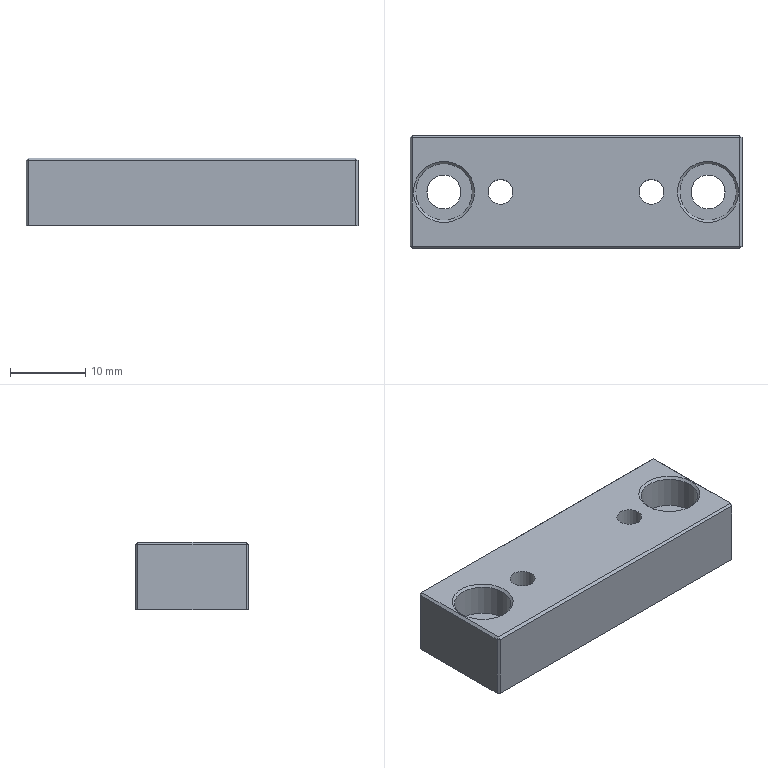Part | NX | 1 solid | 28 faces | box 44 x 15 x 9 mm | volume 5236 mm3 | plane 20 | cylinder 6 | cone 2 | commonest cylinder face diameters 3.3 x2 4.5 x2 7.5 x2
STEP:
#1=CARTESIAN_POINT('',(-106.55,-217.899,185.));
#2=VERTEX_POINT('',#1);
#3=CARTESIAN_POINT('',(-102.5,-217.899,185.));
#4=DIRECTION('',(0.,0.,-1.));
#5=DIRECTION('',(-1.,0.,0.));
#6=AXIS2_PLACEMENT_3D('',#3,#4,#5);
#7=CIRCLE('',#6,4.05);
#8=EDGE_CURVE('',#2,#2,#7,.T.);
#9=ORIENTED_EDGE('',*,*,#8,.F.);
#10=EDGE_LOOP('',(#9));
#11=FACE_BOUND('',#10,.T.);
#12=CARTESIAN_POINT('',(-106.25,-217.899,184.7));
#13=VERTEX_POINT('',#12);
#14=CARTESIAN_POINT('',(-102.5,-217.899,184.7));
#15=DIRECTION('',(0.,0.,1.));
#16=DIRECTION('',(-1.,0.,0.));
#17=AXIS2_PLACEMENT_3D('',#14,#15,#16);
#18=CIRCLE('',#17,3.75);
#19=EDGE_CURVE('',#13,#13,#18,.T.);
#20=ORIENTED_EDGE('',*,*,#19,.F.);
#21=EDGE_LOOP('',(#20));
#22=FACE_BOUND('',#21,.T.);
#23=CARTESIAN_POINT('',(-102.5,-217.899,185.));
#24=DIRECTION('',(0.,0.,1.));
#25=DIRECTION('',(1.,0.,0.));
#26=AXIS2_PLACEMENT_3D('',#23,#24,#25);
#27=CONICAL_SURFACE('',#26,4.05,0.7854);
#28=ADVANCED_FACE('',(#11,#22),#27,.F.);
#29=CARTESIAN_POINT('',(-71.55,-217.899,185.));
#30=VERTEX_POINT('',#29);
#31=CARTESIAN_POINT('',(-67.5,-217.899,185.));
#32=DIRECTION('',(0.,0.,-1.));
#33=DIRECTION('',(-1.,0.,0.));
#34=AXIS2_PLACEMENT_3D('',#31,#32,#33);
#35=CIRCLE('',#34,4.05);
#36=EDGE_CURVE('',#30,#30,#35,.T.);
#37=ORIENTED_EDGE('',*,*,#36,.F.);
#38=EDGE_LOOP('',(#37));
#39=FACE_BOUND('',#38,.T.);
#40=CARTESIAN_POINT('',(-71.25,-217.899,184.7));
#41=VERTEX_POINT('',#40);
#42=CARTESIAN_POINT('',(-67.5,-217.899,184.7));
#43=DIRECTION('',(0.,0.,1.));
#44=DIRECTION('',(-1.,0.,0.));
#45=AXIS2_PLACEMENT_3D('',#42,#43,#44);
#46=CIRCLE('',#45,3.75);
#47=EDGE_CURVE('',#41,#41,#46,.T.);
#48=ORIENTED_EDGE('',*,*,#47,.F.);
#49=EDGE_LOOP('',(#48));
#50=FACE_BOUND('',#49,.T.);
#51=CARTESIAN_POINT('',(-67.5,-217.899,185.));
#52=DIRECTION('',(0.,0.,1.));
#53=DIRECTION('',(1.,0.,0.));
#54=AXIS2_PLACEMENT_3D('',#51,#52,#53);
#55=CONICAL_SURFACE('',#54,4.05,0.7854);
#56=ADVANCED_FACE('',(#39,#50),#55,.F.);
#57=CARTESIAN_POINT('',(-63.,-225.099,184.7));
#58=VERTEX_POINT('',#57);
#59=CARTESIAN_POINT('',(-63.3,-225.399,184.7));
#60=VERTEX_POINT('',#59);
#61=CARTESIAN_POINT('',(-63.3,-225.399,184.7));
#62=DIRECTION('',(-0.7071,-0.7071,0.));
#63=VECTOR('',#62,1000.);
#64=LINE('',#61,#63);
#65=EDGE_CURVE('',#58,#60,#64,.T.);
#66=ORIENTED_EDGE('',*,*,#65,.T.);
#67=CARTESIAN_POINT('',(-63.3,-225.399,176.));
#68=VERTEX_POINT('',#67);
#69=CARTESIAN_POINT('',(-63.3,-225.399,187.));
#70=DIRECTION('',(0.,0.,1.));
#71=VECTOR('',#70,1000.);
#72=LINE('',#69,#71);
#73=EDGE_CURVE('',#68,#60,#72,.T.);
#74=ORIENTED_EDGE('',*,*,#73,.F.);
#75=CARTESIAN_POINT('',(-63.,-225.099,176.));
#76=VERTEX_POINT('',#75);
#77=CARTESIAN_POINT('',(-74.15,-236.249,176.));
#78=DIRECTION('',(-0.7071,-0.7071,0.));
#79=VECTOR('',#78,1000.);
#80=LINE('',#77,#79);
#81=EDGE_CURVE('',#76,#68,#80,.T.);
#82=ORIENTED_EDGE('',*,*,#81,.F.);
#83=CARTESIAN_POINT('',(-63.,-225.099,187.));
#84=DIRECTION('',(0.,0.,-1.));
#85=VECTOR('',#84,1000.);
#86=LINE('',#83,#85);
#87=EDGE_CURVE('',#58,#76,#86,.T.);
#88=ORIENTED_EDGE('',*,*,#87,.F.);
#89=EDGE_LOOP('',(#66,#74,#82,#88));
#90=FACE_BOUND('',#89,.T.);
#91=CARTESIAN_POINT('',(-63.,-225.099,187.));
#92=DIRECTION('',(-0.7071,0.7071,0.));
#93=DIRECTION('',(0.,0.,-1.));
#94=AXIS2_PLACEMENT_3D('',#91,#92,#93);
#95=PLANE('',#94);
#96=ADVANCED_FACE('',(#90),#95,.F.);
#97=CARTESIAN_POINT('',(-63.3,-225.099,185.));
#98=VERTEX_POINT('',#97);
#99=CARTESIAN_POINT('',(-63.15,-225.099,184.85));
#100=DIRECTION('',(-0.7071,0.,0.7071));
#101=VECTOR('',#100,1000.);
#102=LINE('',#99,#101);
#103=EDGE_CURVE('',#58,#98,#102,.T.);
#104=ORIENTED_EDGE('',*,*,#103,.T.);
#105=CARTESIAN_POINT('',(-63.3,-225.399,184.7));
#106=DIRECTION('',(0.,-0.7071,-0.7071));
#107=VECTOR('',#106,1000.);
#108=LINE('',#105,#107);
#109=EDGE_CURVE('',#98,#60,#108,.T.);
#110=ORIENTED_EDGE('',*,*,#109,.T.);
#111=ORIENTED_EDGE('',*,*,#65,.F.);
#112=EDGE_LOOP('',(#104,#110,#111));
#113=FACE_BOUND('',#112,.T.);
#114=CARTESIAN_POINT('',(-63.3,-225.399,184.7));
#115=DIRECTION('',(0.5774,-0.5774,0.5774));
#116=DIRECTION('',(0.7071,0.,-0.7071));
#117=AXIS2_PLACEMENT_3D('',#114,#115,#116);
#118=PLANE('',#117);
#119=ADVANCED_FACE('',(#113),#118,.T.);
#120=CARTESIAN_POINT('',(-63.,-210.699,184.7));
#121=VERTEX_POINT('',#120);
#122=CARTESIAN_POINT('',(-63.3,-210.699,185.));
#123=VERTEX_POINT('',#122);
#124=CARTESIAN_POINT('',(-63.3,-210.699,185.));
#125=DIRECTION('',(-0.7071,0.,0.7071));
#126=VECTOR('',#125,1000.);
#127=LINE('',#124,#126);
#128=EDGE_CURVE('',#121,#123,#127,.T.);
#129=ORIENTED_EDGE('',*,*,#128,.T.);
#130=CARTESIAN_POINT('',(-63.3,-210.399,185.));
#131=DIRECTION('',(0.,1.,0.));
#132=VECTOR('',#131,1000.);
#133=LINE('',#130,#132);
#134=EDGE_CURVE('',#98,#123,#133,.T.);
#135=ORIENTED_EDGE('',*,*,#134,.F.);
#136=ORIENTED_EDGE('',*,*,#103,.F.);
#137=CARTESIAN_POINT('',(-63.,-225.399,184.7));
#138=DIRECTION('',(0.,-1.,0.));
#139=VECTOR('',#138,1000.);
#140=LINE('',#137,#139);
#141=EDGE_CURVE('',#121,#58,#140,.T.);
#142=ORIENTED_EDGE('',*,*,#141,.F.);
#143=EDGE_LOOP('',(#129,#135,#136,#142));
#144=FACE_BOUND('',#143,.T.);
#145=CARTESIAN_POINT('',(-63.,-210.399,184.7));
#146=DIRECTION('',(0.7071,0.,0.7071));
#147=DIRECTION('',(0.,1.,0.));
#148=AXIS2_PLACEMENT_3D('',#145,#146,#147);
#149=PLANE('',#148);
#150=ADVANCED_FACE('',(#144),#149,.T.);
#151=CARTESIAN_POINT('',(-106.7,-225.099,185.));
#152=VERTEX_POINT('',#151);
#153=CARTESIAN_POINT('',(-106.7,-225.399,184.7));
#154=VERTEX_POINT('',#153);
#155=CARTESIAN_POINT('',(-106.7,-225.399,184.7));
#156=DIRECTION('',(0.,-0.7071,-0.7071));
#157=VECTOR('',#156,1000.);
#158=LINE('',#155,#157);
#159=EDGE_CURVE('',#152,#154,#158,.T.);
#160=ORIENTED_EDGE('',*,*,#159,.T.);
#161=CARTESIAN_POINT('',(-107.,-225.399,184.7));
#162=DIRECTION('',(-1.,0.,0.));
#163=VECTOR('',#162,1000.);
#164=LINE('',#161,#163);
#165=EDGE_CURVE('',#60,#154,#164,.T.);
#166=ORIENTED_EDGE('',*,*,#165,.F.);
#167=ORIENTED_EDGE('',*,*,#109,.F.);
#168=CARTESIAN_POINT('',(-63.,-225.099,185.));
#169=DIRECTION('',(1.,0.,0.));
#170=VECTOR('',#169,1000.);
#171=LINE('',#168,#170);
#172=EDGE_CURVE('',#152,#98,#171,.T.);
#173=ORIENTED_EDGE('',*,*,#172,.F.);
#174=EDGE_LOOP('',(#160,#166,#167,#173));
#175=FACE_BOUND('',#174,.T.);
#176=CARTESIAN_POINT('',(-63.,-225.399,184.7));
#177=DIRECTION('',(0.,-0.7071,0.7071));
#178=DIRECTION('',(1.,0.,0.));
#179=AXIS2_PLACEMENT_3D('',#176,#177,#178);
#180=PLANE('',#179);
#181=ADVANCED_FACE('',(#175),#180,.T.);
#182=CARTESIAN_POINT('',(-63.3,-210.399,184.7));
#183=VERTEX_POINT('',#182);
#184=CARTESIAN_POINT('',(-63.15,-210.549,184.7));
#185=DIRECTION('',(-0.7071,0.7071,0.));
#186=VECTOR('',#185,1000.);
#187=LINE('',#184,#186);
#188=EDGE_CURVE('',#121,#183,#187,.T.);
#189=ORIENTED_EDGE('',*,*,#188,.T.);
#190=CARTESIAN_POINT('',(-63.3,-210.699,185.));
#191=DIRECTION('',(0.,-0.7071,0.7071));
#192=VECTOR('',#191,1000.);
#193=LINE('',#190,#192);
#194=EDGE_CURVE('',#183,#123,#193,.T.);
#195=ORIENTED_EDGE('',*,*,#194,.T.);
#196=ORIENTED_EDGE('',*,*,#128,.F.);
#197=EDGE_LOOP('',(#189,#195,#196));
#198=FACE_BOUND('',#197,.T.);
#199=CARTESIAN_POINT('',(-63.3,-210.699,185.));
#200=DIRECTION('',(0.5774,0.5774,0.5774));
#201=DIRECTION('',(0.7071,0.,-0.7071));
#202=AXIS2_PLACEMENT_3D('',#199,#200,#201);
#203=PLANE('',#202);
#204=ADVANCED_FACE('',(#198),#203,.T.);
#205=CARTESIAN_POINT('',(-107.,-225.099,184.7));
#206=VERTEX_POINT('',#205);
#207=CARTESIAN_POINT('',(-106.85,-225.099,184.85));
#208=DIRECTION('',(-0.7071,0.,-0.7071));
#209=VECTOR('',#208,1000.);
#210=LINE('',#207,#209);
#211=EDGE_CURVE('',#152,#206,#210,.T.);
#212=ORIENTED_EDGE('',*,*,#211,.T.);
#213=CARTESIAN_POINT('',(-106.7,-225.399,184.7));
#214=DIRECTION('',(0.7071,-0.7071,0.));
#215=VECTOR('',#214,1000.);
#216=LINE('',#213,#215);
#217=EDGE_CURVE('',#206,#154,#216,.T.);
#218=ORIENTED_EDGE('',*,*,#217,.T.);
#219=ORIENTED_EDGE('',*,*,#159,.F.);
#220=EDGE_LOOP('',(#212,#218,#219));
#221=FACE_BOUND('',#220,.T.);
#222=CARTESIAN_POINT('',(-106.7,-225.399,184.7));
#223=DIRECTION('',(-0.5774,-0.5774,0.5774));
#224=DIRECTION('',(0.7071,0.,0.7071));
#225=AXIS2_PLACEMENT_3D('',#222,#223,#224);
#226=PLANE('',#225);
#227=ADVANCED_FACE('',(#221),#226,.T.);
#228=CARTESIAN_POINT('',(-63.3,-210.399,176.));
#229=VERTEX_POINT('',#228);
#230=CARTESIAN_POINT('',(-63.,-210.699,176.));
#231=VERTEX_POINT('',#230);
#232=CARTESIAN_POINT('',(-66.65,-207.049,176.));
#233=DIRECTION('',(0.7071,-0.7071,0.));
#234=VECTOR('',#233,1000.);
#235=LINE('',#232,#234);
#236=EDGE_CURVE('',#229,#231,#235,.T.);
#237=ORIENTED_EDGE('',*,*,#236,.F.);
#238=CARTESIAN_POINT('',(-63.3,-210.399,187.));
#239=DIRECTION('',(0.,0.,-1.));
#240=VECTOR('',#239,1000.);
#241=LINE('',#238,#240);
#242=EDGE_CURVE('',#183,#229,#241,.T.);
#243=ORIENTED_EDGE('',*,*,#242,.F.);
#244=ORIENTED_EDGE('',*,*,#188,.F.);
#245=CARTESIAN_POINT('',(-63.,-210.699,187.));
#246=DIRECTION('',(0.,0.,1.));
#247=VECTOR('',#246,1000.);
#248=LINE('',#245,#247);
#249=EDGE_CURVE('',#231,#121,#248,.T.);
#250=ORIENTED_EDGE('',*,*,#249,.F.);
#251=EDGE_LOOP('',(#237,#243,#244,#250));
#252=FACE_BOUND('',#251,.T.);
#253=CARTESIAN_POINT('',(-63.3,-210.399,187.));
#254=DIRECTION('',(-0.7071,-0.7071,0.));
#255=DIRECTION('',(0.,0.,-1.));
#256=AXIS2_PLACEMENT_3D('',#253,#254,#255);
#257=PLANE('',#256);
#258=ADVANCED_FACE('',(#252),#257,.F.);
#259=CARTESIAN_POINT('',(-106.7,-210.399,184.7));
#260=VERTEX_POINT('',#259);
#261=CARTESIAN_POINT('',(-106.7,-210.699,185.));
#262=VERTEX_POINT('',#261);
#263=CARTESIAN_POINT('',(-106.7,-210.699,185.));
#264=DIRECTION('',(0.,-0.7071,0.7071));
#265=VECTOR('',#264,1000.);
#266=LINE('',#263,#265);
#267=EDGE_CURVE('',#260,#262,#266,.T.);
#268=ORIENTED_EDGE('',*,*,#267,.T.);
#269=CARTESIAN_POINT('',(-107.,-210.699,185.));
#270=DIRECTION('',(-1.,0.,0.));
#271=VECTOR('',#270,1000.);
#272=LINE('',#269,#271);
#273=EDGE_CURVE('',#123,#262,#272,.T.);
#274=ORIENTED_EDGE('',*,*,#273,.F.);
#275=ORIENTED_EDGE('',*,*,#194,.F.);
#276=CARTESIAN_POINT('',(-63.,-210.399,184.7));
#277=DIRECTION('',(1.,0.,0.));
#278=VECTOR('',#277,1000.);
#279=LINE('',#276,#278);
#280=EDGE_CURVE('',#260,#183,#279,.T.);
#281=ORIENTED_EDGE('',*,*,#280,.F.);
#282=EDGE_LOOP('',(#268,#274,#275,#281));
#283=FACE_BOUND('',#282,.T.);
#284=CARTESIAN_POINT('',(-107.,-210.399,184.7));
#285=DIRECTION('',(0.,0.7071,0.7071));
#286=DIRECTION('',(-1.,0.,0.));
#287=AXIS2_PLACEMENT_3D('',#284,#285,#286);
#288=PLANE('',#287);
#289=ADVANCED_FACE('',(#283),#288,.T.);
#290=CARTESIAN_POINT('',(-107.,-210.699,184.7));
#291=VERTEX_POINT('',#290);
#292=CARTESIAN_POINT('',(-106.7,-210.699,185.));
#293=DIRECTION('',(-0.7071,0.,-0.7071));
#294=VECTOR('',#293,1000.);
#295=LINE('',#292,#294);
#296=EDGE_CURVE('',#262,#291,#295,.T.);
#297=ORIENTED_EDGE('',*,*,#296,.T.);
#298=CARTESIAN_POINT('',(-107.,-210.399,184.7));
#299=DIRECTION('',(0.,1.,0.));
#300=VECTOR('',#299,1000.);
#301=LINE('',#298,#300);
#302=EDGE_CURVE('',#206,#291,#301,.T.);
#303=ORIENTED_EDGE('',*,*,#302,.F.);
#304=ORIENTED_EDGE('',*,*,#211,.F.);
#305=CARTESIAN_POINT('',(-106.7,-225.399,185.));
#306=DIRECTION('',(0.,-1.,0.));
#307=VECTOR('',#306,1000.);
#308=LINE('',#305,#307);
#309=EDGE_CURVE('',#262,#152,#308,.T.);
#310=ORIENTED_EDGE('',*,*,#309,.F.);
#311=EDGE_LOOP('',(#297,#303,#304,#310));
#312=FACE_BOUND('',#311,.T.);
#313=CARTESIAN_POINT('',(-107.,-225.399,184.7));
#314=DIRECTION('',(-0.7071,0.,0.7071));
#315=DIRECTION('',(0.,-1.,0.));
#316=AXIS2_PLACEMENT_3D('',#313,#314,#315);
#317=PLANE('',#316);
#318=ADVANCED_FACE('',(#312),#317,.T.);
#319=CARTESIAN_POINT('',(-106.7,-225.399,176.));
#320=VERTEX_POINT('',#319);
#321=CARTESIAN_POINT('',(-107.,-225.099,176.));
#322=VERTEX_POINT('',#321);
#323=CARTESIAN_POINT('',(-95.85,-236.249,176.));
#324=DIRECTION('',(-0.7071,0.7071,0.));
#325=VECTOR('',#324,1000.);
#326=LINE('',#323,#325);
#327=EDGE_CURVE('',#320,#322,#326,.T.);
#328=ORIENTED_EDGE('',*,*,#327,.F.);
#329=CARTESIAN_POINT('',(-106.7,-225.399,187.));
#330=DIRECTION('',(0.,0.,-1.));
#331=VECTOR('',#330,1000.);
#332=LINE('',#329,#331);
#333=EDGE_CURVE('',#154,#320,#332,.T.);
#334=ORIENTED_EDGE('',*,*,#333,.F.);
#335=ORIENTED_EDGE('',*,*,#217,.F.);
#336=CARTESIAN_POINT('',(-107.,-225.099,187.));
#337=DIRECTION('',(0.,0.,1.));
#338=VECTOR('',#337,1000.);
#339=LINE('',#336,#338);
#340=EDGE_CURVE('',#322,#206,#339,.T.);
#341=ORIENTED_EDGE('',*,*,#340,.F.);
#342=EDGE_LOOP('',(#328,#334,#335,#341));
#343=FACE_BOUND('',#342,.T.);
#344=CARTESIAN_POINT('',(-106.7,-225.399,187.));
#345=DIRECTION('',(0.7071,0.7071,0.));
#346=DIRECTION('',(0.,0.,-1.));
#347=AXIS2_PLACEMENT_3D('',#344,#345,#346);
#348=PLANE('',#347);
#349=ADVANCED_FACE('',(#343),#348,.F.);
#350=ORIENTED_EDGE('',*,*,#267,.F.);
#351=CARTESIAN_POINT('',(-106.85,-210.549,184.7));
#352=DIRECTION('',(-0.7071,-0.7071,0.));
#353=VECTOR('',#352,1000.);
#354=LINE('',#351,#353);
#355=EDGE_CURVE('',#260,#291,#354,.T.);
#356=ORIENTED_EDGE('',*,*,#355,.T.);
#357=ORIENTED_EDGE('',*,*,#296,.F.);
#358=EDGE_LOOP('',(#350,#356,#357));
#359=FACE_BOUND('',#358,.T.);
#360=CARTESIAN_POINT('',(-106.7,-210.699,185.));
#361=DIRECTION('',(-0.5774,0.5774,0.5774));
#362=DIRECTION('',(0.7071,0.,0.7071));
#363=AXIS2_PLACEMENT_3D('',#360,#361,#362);
#364=PLANE('',#363);
#365=ADVANCED_FACE('',(#359),#364,.T.);
#366=ORIENTED_EDGE('',*,*,#355,.F.);
#367=CARTESIAN_POINT('',(-106.7,-210.399,176.));
#368=VERTEX_POINT('',#367);
#369=CARTESIAN_POINT('',(-106.7,-210.399,187.));
#370=DIRECTION('',(0.,0.,1.));
#371=VECTOR('',#370,1000.);
#372=LINE('',#369,#371);
#373=EDGE_CURVE('',#368,#260,#372,.T.);
#374=ORIENTED_EDGE('',*,*,#373,.F.);
#375=CARTESIAN_POINT('',(-107.,-210.699,176.));
#376=VERTEX_POINT('',#375);
#377=CARTESIAN_POINT('',(-103.35,-207.049,176.));
#378=DIRECTION('',(0.7071,0.7071,0.));
#379=VECTOR('',#378,1000.);
#380=LINE('',#377,#379);
#381=EDGE_CURVE('',#376,#368,#380,.T.);
#382=ORIENTED_EDGE('',*,*,#381,.F.);
#383=CARTESIAN_POINT('',(-107.,-210.699,187.));
#384=DIRECTION('',(0.,0.,-1.));
#385=VECTOR('',#384,1000.);
#386=LINE('',#383,#385);
#387=EDGE_CURVE('',#291,#376,#386,.T.);
#388=ORIENTED_EDGE('',*,*,#387,.F.);
#389=EDGE_LOOP('',(#366,#374,#382,#388));
#390=FACE_BOUND('',#389,.T.);
#391=CARTESIAN_POINT('',(-107.,-210.699,187.));
#392=DIRECTION('',(0.7071,-0.7071,0.));
#393=DIRECTION('',(0.,0.,-1.));
#394=AXIS2_PLACEMENT_3D('',#391,#392,#393);
#395=PLANE('',#394);
#396=ADVANCED_FACE('',(#390),#395,.F.);
#397=CARTESIAN_POINT('',(-76.65,-217.899,185.));
#398=VERTEX_POINT('',#397);
#399=CARTESIAN_POINT('',(-75.,-217.899,185.));
#400=DIRECTION('',(0.,0.,1.));
#401=DIRECTION('',(-1.,0.,0.));
#402=AXIS2_PLACEMENT_3D('',#399,#400,#401);
#403=CIRCLE('',#402,1.65);
#404=EDGE_CURVE('',#398,#398,#403,.T.);
#405=ORIENTED_EDGE('',*,*,#404,.T.);
#406=EDGE_LOOP('',(#405));
#407=FACE_BOUND('',#406,.T.);
#408=CARTESIAN_POINT('',(-73.35,-217.899,176.));
#409=VERTEX_POINT('',#408);
#410=CARTESIAN_POINT('',(-75.,-217.899,176.));
#411=DIRECTION('',(0.,0.,-1.));
#412=DIRECTION('',(1.,0.,0.));
#413=AXIS2_PLACEMENT_3D('',#410,#411,#412);
#414=CIRCLE('',#413,1.65);
#415=EDGE_CURVE('',#409,#409,#414,.T.);
#416=ORIENTED_EDGE('',*,*,#415,.T.);
#417=EDGE_LOOP('',(#416));
#418=FACE_BOUND('',#417,.T.);
#419=CARTESIAN_POINT('',(-75.,-217.899,185.));
#420=DIRECTION('',(0.,0.,-1.));
#421=DIRECTION('',(-1.,0.,0.));
#422=AXIS2_PLACEMENT_3D('',#419,#420,#421);
#423=CYLINDRICAL_SURFACE('',#422,1.65);
#424=ADVANCED_FACE('',(#407,#418),#423,.F.);
#425=CARTESIAN_POINT('',(-93.35,-217.899,185.));
#426=VERTEX_POINT('',#425);
#427=CARTESIAN_POINT('',(-95.,-217.899,185.));
#428=DIRECTION('',(0.,0.,-1.));
#429=DIRECTION('',(1.,0.,0.));
#430=AXIS2_PLACEMENT_3D('',#427,#428,#429);
#431=CIRCLE('',#430,1.65);
#432=EDGE_CURVE('',#426,#426,#431,.T.);
#433=ORIENTED_EDGE('',*,*,#432,.F.);
#434=EDGE_LOOP('',(#433));
#435=FACE_BOUND('',#434,.T.);
#436=CARTESIAN_POINT('',(-96.65,-217.899,176.));
#437=VERTEX_POINT('',#436);
#438=CARTESIAN_POINT('',(-95.,-217.899,176.));
#439=DIRECTION('',(0.,0.,1.));
#440=DIRECTION('',(-1.,0.,0.));
#441=AXIS2_PLACEMENT_3D('',#438,#439,#440);
#442=CIRCLE('',#441,1.65);
#443=EDGE_CURVE('',#437,#437,#442,.T.);
#444=ORIENTED_EDGE('',*,*,#443,.F.);
#445=EDGE_LOOP('',(#444));
#446=FACE_BOUND('',#445,.T.);
#447=CARTESIAN_POINT('',(-95.,-217.899,185.));
#448=DIRECTION('',(0.,0.,-1.));
#449=DIRECTION('',(1.,0.,0.));
#450=AXIS2_PLACEMENT_3D('',#447,#448,#449);
#451=CYLINDRICAL_SURFACE('',#450,1.65);
#452=ADVANCED_FACE('',(#435,#446),#451,.F.);
#453=CARTESIAN_POINT('',(-71.25,-217.899,180.5));
#454=VERTEX_POINT('',#453);
#455=CARTESIAN_POINT('',(-67.5,-217.899,180.5));
#456=DIRECTION('',(0.,0.,-1.));
#457=DIRECTION('',(-1.,0.,0.));
#458=AXIS2_PLACEMENT_3D('',#455,#456,#457);
#459=CIRCLE('',#458,3.75);
#460=EDGE_CURVE('',#454,#454,#459,.T.);
#461=ORIENTED_EDGE('',*,*,#460,.T.);
#462=EDGE_LOOP('',(#461));
#463=FACE_BOUND('',#462,.T.);
#464=ORIENTED_EDGE('',*,*,#47,.T.);
#465=EDGE_LOOP('',(#464));
#466=FACE_BOUND('',#465,.T.);
#467=CARTESIAN_POINT('',(-67.5,-217.899,185.));
#468=DIRECTION('',(0.,0.,-1.));
#469=DIRECTION('',(1.,0.,0.));
#470=AXIS2_PLACEMENT_3D('',#467,#468,#469);
#471=CYLINDRICAL_SURFACE('',#470,3.75);
#472=ADVANCED_FACE('',(#463,#466),#471,.F.);
#473=CARTESIAN_POINT('',(-69.75,-217.899,180.5));
#474=VERTEX_POINT('',#473);
#475=CARTESIAN_POINT('',(-67.5,-217.899,180.5));
#476=DIRECTION('',(0.,0.,1.));
#477=DIRECTION('',(-1.,0.,0.));
#478=AXIS2_PLACEMENT_3D('',#475,#476,#477);
#479=CIRCLE('',#478,2.25);
#480=EDGE_CURVE('',#474,#474,#479,.T.);
#481=ORIENTED_EDGE('',*,*,#480,.F.);
#482=EDGE_LOOP('',(#481));
#483=FACE_BOUND('',#482,.T.);
#484=ORIENTED_EDGE('',*,*,#460,.F.);
#485=EDGE_LOOP('',(#484));
#486=FACE_BOUND('',#485,.T.);
#487=CARTESIAN_POINT('',(-102.5,-217.899,180.5));
#488=DIRECTION('',(0.,0.,-1.));
#489=DIRECTION('',(-1.,0.,0.));
#490=AXIS2_PLACEMENT_3D('',#487,#488,#489);
#491=PLANE('',#490);
#492=ADVANCED_FACE('',(#483,#486),#491,.F.);
#493=CARTESIAN_POINT('',(-98.75,-217.899,180.5));
#494=VERTEX_POINT('',#493);
#495=CARTESIAN_POINT('',(-102.5,-217.899,180.5));
#496=DIRECTION('',(0.,0.,-1.));
#497=DIRECTION('',(1.,0.,0.));
#498=AXIS2_PLACEMENT_3D('',#495,#496,#497);
#499=CIRCLE('',#498,3.75);
#500=EDGE_CURVE('',#494,#494,#499,.T.);
#501=ORIENTED_EDGE('',*,*,#500,.T.);
#502=EDGE_LOOP('',(#501));
#503=FACE_BOUND('',#502,.T.);
#504=ORIENTED_EDGE('',*,*,#19,.T.);
#505=EDGE_LOOP('',(#504));
#506=FACE_BOUND('',#505,.T.);
#507=CARTESIAN_POINT('',(-102.5,-217.899,185.));
#508=DIRECTION('',(0.,0.,-1.));
#509=DIRECTION('',(1.,0.,0.));
#510=AXIS2_PLACEMENT_3D('',#507,#508,#509);
#511=CYLINDRICAL_SURFACE('',#510,3.75);
#512=ADVANCED_FACE('',(#503,#506),#511,.F.);
#513=CARTESIAN_POINT('',(-104.75,-217.899,180.5));
#514=VERTEX_POINT('',#513);
#515=CARTESIAN_POINT('',(-102.5,-217.899,180.5));
#516=DIRECTION('',(0.,0.,1.));
#517=DIRECTION('',(-1.,0.,0.));
#518=AXIS2_PLACEMENT_3D('',#515,#516,#517);
#519=CIRCLE('',#518,2.25);
#520=EDGE_CURVE('',#514,#514,#519,.T.);
#521=ORIENTED_EDGE('',*,*,#520,.F.);
#522=EDGE_LOOP('',(#521));
#523=FACE_BOUND('',#522,.T.);
#524=ORIENTED_EDGE('',*,*,#500,.F.);
#525=EDGE_LOOP('',(#524));
#526=FACE_BOUND('',#525,.T.);
#527=CARTESIAN_POINT('',(-102.5,-217.899,180.5));
#528=DIRECTION('',(0.,0.,-1.));
#529=DIRECTION('',(-1.,0.,0.));
#530=AXIS2_PLACEMENT_3D('',#527,#528,#529);
#531=PLANE('',#530);
#532=ADVANCED_FACE('',(#523,#526),#531,.F.);
#533=CARTESIAN_POINT('',(-69.75,-217.899,176.));
#534=VERTEX_POINT('',#533);
#535=CARTESIAN_POINT('',(-67.5,-217.899,176.));
#536=DIRECTION('',(0.,0.,-1.));
#537=DIRECTION('',(-1.,0.,0.));
#538=AXIS2_PLACEMENT_3D('',#535,#536,#537);
#539=CIRCLE('',#538,2.25);
#540=EDGE_CURVE('',#534,#534,#539,.T.);
#541=ORIENTED_EDGE('',*,*,#540,.T.);
#542=EDGE_LOOP('',(#541));
#543=FACE_BOUND('',#542,.T.);
#544=ORIENTED_EDGE('',*,*,#480,.T.);
#545=EDGE_LOOP('',(#544));
#546=FACE_BOUND('',#545,.T.);
#547=CARTESIAN_POINT('',(-67.5,-217.899,187.));
#548=DIRECTION('',(0.,0.,-1.));
#549=DIRECTION('',(1.,0.,0.));
#550=AXIS2_PLACEMENT_3D('',#547,#548,#549);
#551=CYLINDRICAL_SURFACE('',#550,2.25);
#552=ADVANCED_FACE('',(#543,#546),#551,.F.);
#553=CARTESIAN_POINT('',(-104.75,-217.899,176.));
#554=VERTEX_POINT('',#553);
#555=CARTESIAN_POINT('',(-102.5,-217.899,176.));
#556=DIRECTION('',(0.,0.,-1.));
#557=DIRECTION('',(-1.,0.,0.));
#558=AXIS2_PLACEMENT_3D('',#555,#556,#557);
#559=CIRCLE('',#558,2.25);
#560=EDGE_CURVE('',#554,#554,#559,.T.);
#561=ORIENTED_EDGE('',*,*,#560,.T.);
#562=EDGE_LOOP('',(#561));
#563=FACE_BOUND('',#562,.T.);
#564=ORIENTED_EDGE('',*,*,#520,.T.);
#565=EDGE_LOOP('',(#564));
#566=FACE_BOUND('',#565,.T.);
#567=CARTESIAN_POINT('',(-102.5,-217.899,187.));
#568=DIRECTION('',(0.,0.,-1.));
#569=DIRECTION('',(1.,0.,0.));
#570=AXIS2_PLACEMENT_3D('',#567,#568,#569);
#571=CYLINDRICAL_SURFACE('',#570,2.25);
#572=ADVANCED_FACE('',(#563,#566),#571,.F.);
#573=CARTESIAN_POINT('',(-63.,-210.399,176.));
#574=DIRECTION('',(0.,-1.,0.));
#575=VECTOR('',#574,1000.);
#576=LINE('',#573,#575);
#577=EDGE_CURVE('',#231,#76,#576,.T.);
#578=ORIENTED_EDGE('',*,*,#577,.T.);
#579=ORIENTED_EDGE('',*,*,#81,.T.);
#580=CARTESIAN_POINT('',(-63.,-225.399,176.));
#581=DIRECTION('',(-1.,0.,0.));
#582=VECTOR('',#581,1000.);
#583=LINE('',#580,#582);
#584=EDGE_CURVE('',#68,#320,#583,.T.);
#585=ORIENTED_EDGE('',*,*,#584,.T.);
#586=ORIENTED_EDGE('',*,*,#327,.T.);
#587=CARTESIAN_POINT('',(-107.,-225.399,176.));
#588=DIRECTION('',(0.,1.,0.));
#589=VECTOR('',#588,1000.);
#590=LINE('',#587,#589);
#591=EDGE_CURVE('',#322,#376,#590,.T.);
#592=ORIENTED_EDGE('',*,*,#591,.T.);
#593=ORIENTED_EDGE('',*,*,#381,.T.);
#594=CARTESIAN_POINT('',(-107.,-210.399,176.));
#595=DIRECTION('',(1.,0.,0.));
#596=VECTOR('',#595,1000.);
#597=LINE('',#594,#596);
#598=EDGE_CURVE('',#368,#229,#597,.T.);
#599=ORIENTED_EDGE('',*,*,#598,.T.);
#600=ORIENTED_EDGE('',*,*,#236,.T.);
#601=EDGE_LOOP('',(#578,#579,#585,#586,#592,#593,#599,#600));
#602=FACE_BOUND('',#601,.T.);
#603=ORIENTED_EDGE('',*,*,#560,.F.);
#604=EDGE_LOOP('',(#603));
#605=FACE_BOUND('',#604,.T.);
#606=ORIENTED_EDGE('',*,*,#540,.F.);
#607=EDGE_LOOP('',(#606));
#608=FACE_BOUND('',#607,.T.);
#609=ORIENTED_EDGE('',*,*,#443,.T.);
#610=EDGE_LOOP('',(#609));
#611=FACE_BOUND('',#610,.T.);
#612=ORIENTED_EDGE('',*,*,#415,.F.);
#613=EDGE_LOOP('',(#612));
#614=FACE_BOUND('',#613,.T.);
#615=CARTESIAN_POINT('',(-85.,-225.399,176.));
#616=DIRECTION('',(0.,0.,-1.));
#617=DIRECTION('',(1.,0.,0.));
#618=AXIS2_PLACEMENT_3D('',#615,#616,#617);
#619=PLANE('',#618);
#620=ADVANCED_FACE('',(#602,#605,#608,#611,#614),#619,.T.);
#621=ORIENTED_EDGE('',*,*,#432,.T.);
#622=EDGE_LOOP('',(#621));
#623=FACE_BOUND('',#622,.T.);
#624=ORIENTED_EDGE('',*,*,#404,.F.);
#625=EDGE_LOOP('',(#624));
#626=FACE_BOUND('',#625,.T.);
#627=ORIENTED_EDGE('',*,*,#8,.T.);
#628=EDGE_LOOP('',(#627));
#629=FACE_BOUND('',#628,.T.);
#630=ORIENTED_EDGE('',*,*,#172,.T.);
#631=ORIENTED_EDGE('',*,*,#134,.T.);
#632=ORIENTED_EDGE('',*,*,#273,.T.);
#633=ORIENTED_EDGE('',*,*,#309,.T.);
#634=EDGE_LOOP('',(#630,#631,#632,#633));
#635=FACE_BOUND('',#634,.T.);
#636=ORIENTED_EDGE('',*,*,#36,.T.);
#637=EDGE_LOOP('',(#636));
#638=FACE_BOUND('',#637,.T.);
#639=CARTESIAN_POINT('',(-85.,-225.399,185.));
#640=DIRECTION('',(0.,0.,-1.));
#641=DIRECTION('',(1.,0.,0.));
#642=AXIS2_PLACEMENT_3D('',#639,#640,#641);
#643=PLANE('',#642);
#644=ADVANCED_FACE('',(#623,#626,#629,#635,#638),#643,.F.);
#645=ORIENTED_EDGE('',*,*,#141,.T.);
#646=ORIENTED_EDGE('',*,*,#87,.T.);
#647=ORIENTED_EDGE('',*,*,#577,.F.);
#648=ORIENTED_EDGE('',*,*,#249,.T.);
#649=EDGE_LOOP('',(#645,#646,#647,#648));
#650=FACE_BOUND('',#649,.T.);
#651=CARTESIAN_POINT('',(-63.,-210.399,187.));
#652=DIRECTION('',(1.,0.,0.));
#653=DIRECTION('',(0.,0.,-1.));
#654=AXIS2_PLACEMENT_3D('',#651,#652,#653);
#655=PLANE('',#654);
#656=ADVANCED_FACE('',(#650),#655,.T.);
#657=ORIENTED_EDGE('',*,*,#584,.F.);
#658=ORIENTED_EDGE('',*,*,#73,.T.);
#659=ORIENTED_EDGE('',*,*,#165,.T.);
#660=ORIENTED_EDGE('',*,*,#333,.T.);
#661=EDGE_LOOP('',(#657,#658,#659,#660));
#662=FACE_BOUND('',#661,.T.);
#663=CARTESIAN_POINT('',(-63.,-225.399,187.));
#664=DIRECTION('',(0.,-1.,0.));
#665=DIRECTION('',(0.,0.,-1.));
#666=AXIS2_PLACEMENT_3D('',#663,#664,#665);
#667=PLANE('',#666);
#668=ADVANCED_FACE('',(#662),#667,.T.);
#669=ORIENTED_EDGE('',*,*,#591,.F.);
#670=ORIENTED_EDGE('',*,*,#340,.T.);
#671=ORIENTED_EDGE('',*,*,#302,.T.);
#672=ORIENTED_EDGE('',*,*,#387,.T.);
#673=EDGE_LOOP('',(#669,#670,#671,#672));
#674=FACE_BOUND('',#673,.T.);
#675=CARTESIAN_POINT('',(-107.,-225.399,187.));
#676=DIRECTION('',(-1.,0.,0.));
#677=DIRECTION('',(0.,0.,1.));
#678=AXIS2_PLACEMENT_3D('',#675,#676,#677);
#679=PLANE('',#678);
#680=ADVANCED_FACE('',(#674),#679,.T.);
#681=ORIENTED_EDGE('',*,*,#280,.T.);
#682=ORIENTED_EDGE('',*,*,#242,.T.);
#683=ORIENTED_EDGE('',*,*,#598,.F.);
#684=ORIENTED_EDGE('',*,*,#373,.T.);
#685=EDGE_LOOP('',(#681,#682,#683,#684));
#686=FACE_BOUND('',#685,.T.);
#687=CARTESIAN_POINT('',(-107.,-210.399,187.));
#688=DIRECTION('',(0.,1.,0.));
#689=DIRECTION('',(0.,0.,1.));
#690=AXIS2_PLACEMENT_3D('',#687,#688,#689);
#691=PLANE('',#690);
#692=ADVANCED_FACE('',(#686),#691,.T.);
#693=CLOSED_SHELL('',(#28,#56,#96,#119,#150,#181,#204,#227,#258,#289,#318,#349,#365,#396,#424,#452,#472,#492,#512,#532,#552,#572,#620,#644,#656,#668,#680,#692));
#694=MANIFOLD_SOLID_BREP('',#693);
#695=(LENGTH_UNIT()NAMED_UNIT(*)SI_UNIT(.MILLI.,.METRE.));
#696=UNCERTAINTY_MEASURE_WITH_UNIT(LENGTH_MEASURE(0.00001),#695,'','');
#697=(NAMED_UNIT(*)PLANE_ANGLE_UNIT()SI_UNIT($,.RADIAN.));
#698=(NAMED_UNIT(*)SI_UNIT($,.STERADIAN.)SOLID_ANGLE_UNIT());
#699=(GEOMETRIC_REPRESENTATION_CONTEXT(3)GLOBAL_UNCERTAINTY_ASSIGNED_CONTEXT((#696))GLOBAL_UNIT_ASSIGNED_CONTEXT((#695,#697,#698))REPRESENTATION_CONTEXT('',''));
#700=ADVANCED_BREP_SHAPE_REPRESENTATION('',(#694),#699);